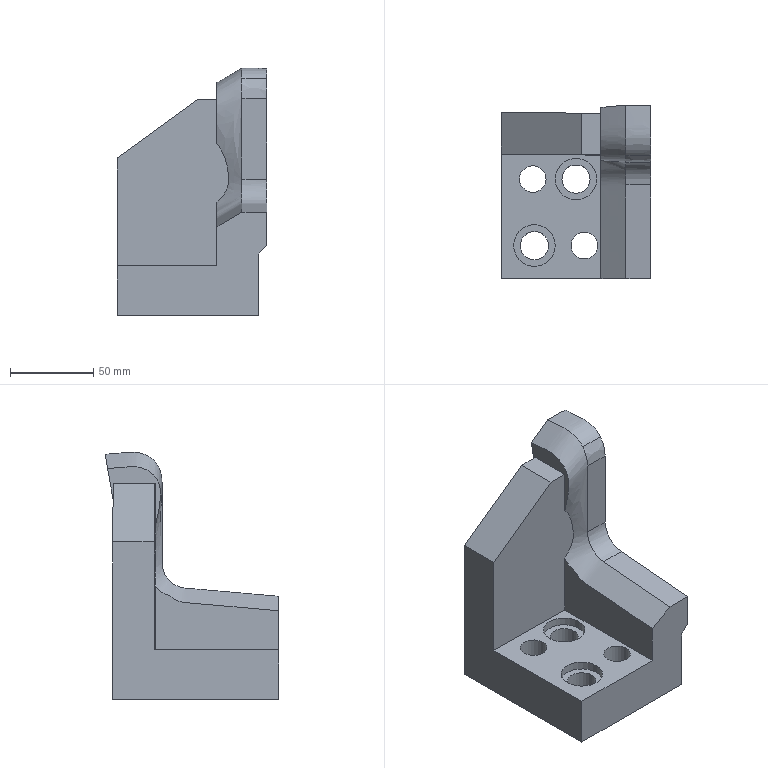Part | NX | features solid 2 | 1 solid | 29 faces | box 90 x 104.296 x 148.805 mm | volume 514117 mm3 | spline 12 | plane 11 | cylinder 6 | commonest cylinder face diameters 16 x2 17 x2 25 x2